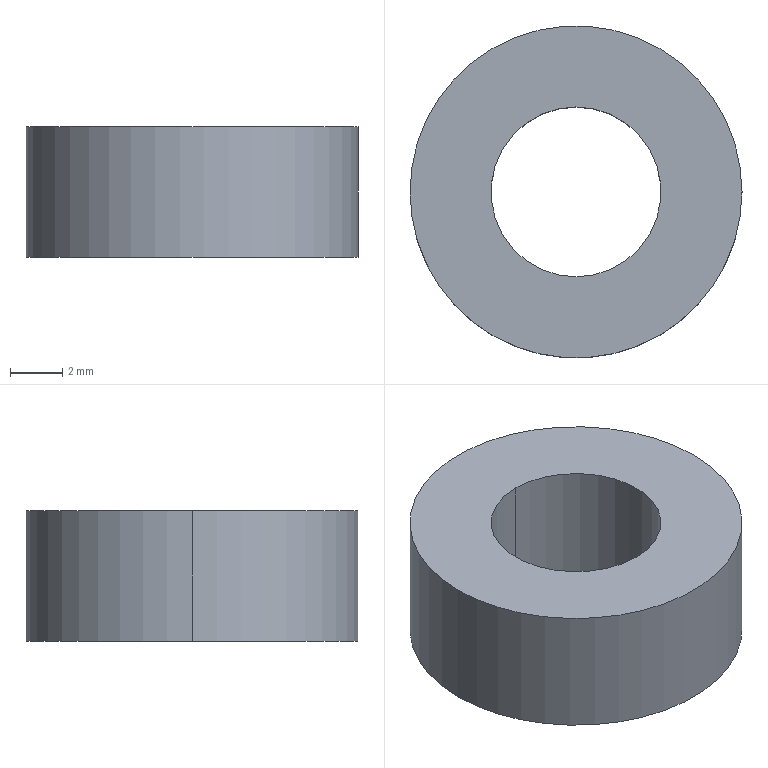Part | STEP file | 1_id1470_x_t | 1 solid | 6 faces | box 12.7 x 12.7 x 5 mm | volume 467.469 mm3 | cylinder 4 | plane 2 | commonest cylinder face diameters 6.5 x2 12.7 x2
STEP:
#1=CARTESIAN_POINT('',(0.,0.,0.));
#2=DIRECTION('',(0.,0.,1.));
#3=DIRECTION('',(1.,0.,0.));
#4=AXIS2_PLACEMENT_3D('',#1,#2,#3);
#5=CARTESIAN_POINT('',(928.809,131.395,-85.));
#6=VERTEX_POINT('',#5);
#7=CARTESIAN_POINT('',(928.809,137.895,-85.));
#8=VERTEX_POINT('',#7);
#9=CARTESIAN_POINT('',(928.809,134.645,-85.));
#10=DIRECTION('',(0.,0.,1.));
#11=DIRECTION('',(0.,-1.,0.));
#12=AXIS2_PLACEMENT_3D('',#9,#10,#11);
#13=CIRCLE('',#12,3.25);
#14=CARTESIAN_POINT('',(928.809,134.645,-88.25));
#15=DIRECTION('',(0.,0.,-1.));
#16=DIRECTION('',(0.,-1.,0.));
#17=AXIS2_PLACEMENT_3D('',#14,#15,#16);
#18=CYLINDRICAL_SURFACE('',#17,3.25);
#19=CARTESIAN_POINT('',(6.283,-3.25));
#20=DIRECTION('',(-1.,0.));
#21=VECTOR('',#20,1.);
#22=LINE('',#19,#21);
#23=(GEOMETRIC_REPRESENTATION_CONTEXT(2)PARAMETRIC_REPRESENTATION_CONTEXT()REPRESENTATION_CONTEXT('',''));
#24=DEFINITIONAL_REPRESENTATION('',(#22),#23);
#25=PCURVE('',#18,#24);
#26=CARTESIAN_POINT('',(928.809,134.645,-85.));
#27=DIRECTION('',(0.,0.,1.));
#28=DIRECTION('',(0.,-1.,0.));
#29=AXIS2_PLACEMENT_3D('',#26,#27,#28);
#30=PLANE('',#29);
#31=CARTESIAN_POINT('',(0.,0.));
#32=DIRECTION('',(1.,0.));
#33=AXIS2_PLACEMENT_2D('',#31,#32);
#34=CIRCLE('',#33,3.25);
#35=(GEOMETRIC_REPRESENTATION_CONTEXT(2)PARAMETRIC_REPRESENTATION_CONTEXT()REPRESENTATION_CONTEXT('',''));
#36=DEFINITIONAL_REPRESENTATION('',(#34),#35);
#37=PCURVE('',#30,#36);
#38=SURFACE_CURVE('',#13,(#25,#37),.PCURVE_S1.);
#39=EDGE_CURVE('',#6,#8,#38,.T.);
#40=ORIENTED_EDGE('',*,*,#39,.T.);
#41=CARTESIAN_POINT('',(928.809,137.895,-80.));
#42=VERTEX_POINT('',#41);
#43=CARTESIAN_POINT('',(928.809,137.895,-80.));
#44=DIRECTION('',(0.,0.,1.));
#45=VECTOR('',#44,1.);
#46=LINE('',#43,#45);
#47=CARTESIAN_POINT('',(3.142,-8.25));
#48=DIRECTION('',(0.,-1.));
#49=VECTOR('',#48,1.);
#50=LINE('',#47,#49);
#51=(GEOMETRIC_REPRESENTATION_CONTEXT(2)PARAMETRIC_REPRESENTATION_CONTEXT()REPRESENTATION_CONTEXT('',''));
#52=DEFINITIONAL_REPRESENTATION('',(#50),#51);
#53=PCURVE('',#18,#52);
#54=CARTESIAN_POINT('',(928.809,134.645,-88.25));
#55=DIRECTION('',(0.,0.,-1.));
#56=DIRECTION('',(0.,-1.,0.));
#57=AXIS2_PLACEMENT_3D('',#54,#55,#56);
#58=CYLINDRICAL_SURFACE('',#57,3.25);
#59=CARTESIAN_POINT('',(3.142,-8.25));
#60=DIRECTION('',(0.,-1.));
#61=VECTOR('',#60,1.);
#62=LINE('',#59,#61);
#63=(GEOMETRIC_REPRESENTATION_CONTEXT(2)PARAMETRIC_REPRESENTATION_CONTEXT()REPRESENTATION_CONTEXT('',''));
#64=DEFINITIONAL_REPRESENTATION('',(#62),#63);
#65=PCURVE('',#58,#64);
#66=SURFACE_CURVE('',#46,(#53,#65),.PCURVE_S1.);
#67=EDGE_CURVE('',#8,#42,#66,.T.);
#68=ORIENTED_EDGE('',*,*,#67,.T.);
#69=CARTESIAN_POINT('',(928.809,131.395,-80.));
#70=VERTEX_POINT('',#69);
#71=CARTESIAN_POINT('',(928.809,134.645,-80.));
#72=DIRECTION('',(0.,0.,-1.));
#73=DIRECTION('',(0.,1.,0.));
#74=AXIS2_PLACEMENT_3D('',#71,#72,#73);
#75=CIRCLE('',#74,3.25);
#76=CARTESIAN_POINT('',(3.142,-8.25));
#77=DIRECTION('',(1.,0.));
#78=VECTOR('',#77,1.);
#79=LINE('',#76,#78);
#80=(GEOMETRIC_REPRESENTATION_CONTEXT(2)PARAMETRIC_REPRESENTATION_CONTEXT()REPRESENTATION_CONTEXT('',''));
#81=DEFINITIONAL_REPRESENTATION('',(#79),#80);
#82=PCURVE('',#18,#81);
#83=CARTESIAN_POINT('',(928.809,134.645,-80.));
#84=DIRECTION('',(0.,0.,1.));
#85=DIRECTION('',(0.,-1.,0.));
#86=AXIS2_PLACEMENT_3D('',#83,#84,#85);
#87=PLANE('',#86);
#88=CARTESIAN_POINT('',(-3.25,0.));
#89=CARTESIAN_POINT('',(-3.25,5.629));
#90=CARTESIAN_POINT('',(1.625,2.815));
#91=CARTESIAN_POINT('',(6.5,0.));
#92=CARTESIAN_POINT('',(1.625,-2.815));
#93=CARTESIAN_POINT('',(-3.25,-5.629));
#94=CARTESIAN_POINT('',(-3.25,0.));
#95=(BOUNDED_CURVE()B_SPLINE_CURVE(2,(#88,#89,#90,#91,#92,#93,#94),.UNSPECIFIED.,.T.,.F.)B_SPLINE_CURVE_WITH_KNOTS((1,2,2,2,2,1),(-2.094,0.,2.094,4.189,6.283,8.378),.UNSPECIFIED.)CURVE()GEOMETRIC_REPRESENTATION_ITEM()RATIONAL_B_SPLINE_CURVE((1.,0.5,1.,0.5,1.,0.5,1.))REPRESENTATION_ITEM(''));
#96=(GEOMETRIC_REPRESENTATION_CONTEXT(2)PARAMETRIC_REPRESENTATION_CONTEXT()REPRESENTATION_CONTEXT('',''));
#97=DEFINITIONAL_REPRESENTATION('',(#95),#96);
#98=PCURVE('',#87,#97);
#99=SURFACE_CURVE('',#75,(#82,#98),.PCURVE_S1.);
#100=EDGE_CURVE('',#42,#70,#99,.T.);
#101=ORIENTED_EDGE('',*,*,#100,.T.);
#102=CARTESIAN_POINT('',(928.809,131.395,-80.));
#103=DIRECTION('',(0.,0.,-1.));
#104=VECTOR('',#103,1.);
#105=LINE('',#102,#104);
#106=CARTESIAN_POINT('',(6.283,-8.25));
#107=DIRECTION('',(0.,1.));
#108=VECTOR('',#107,1.);
#109=LINE('',#106,#108);
#110=(GEOMETRIC_REPRESENTATION_CONTEXT(2)PARAMETRIC_REPRESENTATION_CONTEXT()REPRESENTATION_CONTEXT('',''));
#111=DEFINITIONAL_REPRESENTATION('',(#109),#110);
#112=PCURVE('',#18,#111);
#113=CARTESIAN_POINT('',(0.,-8.25));
#114=DIRECTION('',(0.,1.));
#115=VECTOR('',#114,1.);
#116=LINE('',#113,#115);
#117=(GEOMETRIC_REPRESENTATION_CONTEXT(2)PARAMETRIC_REPRESENTATION_CONTEXT()REPRESENTATION_CONTEXT('',''));
#118=DEFINITIONAL_REPRESENTATION('',(#116),#117);
#119=PCURVE('',#58,#118);
#120=SURFACE_CURVE('',#105,(#112,#119),.PCURVE_S1.);
#121=EDGE_CURVE('',#70,#6,#120,.T.);
#122=ORIENTED_EDGE('',*,*,#121,.T.);
#123=EDGE_LOOP('',(#40,#68,#101,#122));
#124=FACE_BOUND('',#123,.F.);
#125=ADVANCED_FACE('',(#124),#18,.F.);
#126=CARTESIAN_POINT('',(922.459,134.645,-85.));
#127=VERTEX_POINT('',#126);
#128=CARTESIAN_POINT('',(935.159,134.645,-85.));
#129=VERTEX_POINT('',#128);
#130=CARTESIAN_POINT('',(928.809,134.645,-85.));
#131=DIRECTION('',(0.,0.,-1.));
#132=DIRECTION('',(-1.,0.,0.));
#133=AXIS2_PLACEMENT_3D('',#130,#131,#132);
#134=CIRCLE('',#133,6.35);
#135=CARTESIAN_POINT('',(0.,-6.35));
#136=CARTESIAN_POINT('',(-10.999,-6.35));
#137=CARTESIAN_POINT('',(-5.499,3.175));
#138=CARTESIAN_POINT('',(0.,12.7));
#139=CARTESIAN_POINT('',(5.499,3.175));
#140=CARTESIAN_POINT('',(10.999,-6.35));
#141=CARTESIAN_POINT('',(0.,-6.35));
#142=(BOUNDED_CURVE()B_SPLINE_CURVE(2,(#135,#136,#137,#138,#139,#140,#141),.UNSPECIFIED.,.T.,.F.)B_SPLINE_CURVE_WITH_KNOTS((1,2,2,2,2,1),(-2.094,0.,2.094,4.189,6.283,8.378),.UNSPECIFIED.)CURVE()GEOMETRIC_REPRESENTATION_ITEM()RATIONAL_B_SPLINE_CURVE((1.,0.5,1.,0.5,1.,0.5,1.))REPRESENTATION_ITEM(''));
#143=(GEOMETRIC_REPRESENTATION_CONTEXT(2)PARAMETRIC_REPRESENTATION_CONTEXT()REPRESENTATION_CONTEXT('',''));
#144=DEFINITIONAL_REPRESENTATION('',(#142),#143);
#145=PCURVE('',#30,#144);
#146=CARTESIAN_POINT('',(928.809,134.645,-80.));
#147=DIRECTION('',(0.,0.,1.));
#148=DIRECTION('',(1.,0.,0.));
#149=AXIS2_PLACEMENT_3D('',#146,#147,#148);
#150=CYLINDRICAL_SURFACE('',#149,6.35);
#151=CARTESIAN_POINT('',(3.142,-5.));
#152=DIRECTION('',(-1.,0.));
#153=VECTOR('',#152,1.);
#154=LINE('',#151,#153);
#155=(GEOMETRIC_REPRESENTATION_CONTEXT(2)PARAMETRIC_REPRESENTATION_CONTEXT()REPRESENTATION_CONTEXT('',''));
#156=DEFINITIONAL_REPRESENTATION('',(#154),#155);
#157=PCURVE('',#150,#156);
#158=SURFACE_CURVE('',#134,(#145,#157),.PCURVE_S1.);
#159=EDGE_CURVE('',#127,#129,#158,.T.);
#160=ORIENTED_EDGE('',*,*,#159,.T.);
#161=CARTESIAN_POINT('',(928.809,134.645,-85.));
#162=DIRECTION('',(0.,0.,-1.));
#163=DIRECTION('',(1.,0.,0.));
#164=AXIS2_PLACEMENT_3D('',#161,#162,#163);
#165=CIRCLE('',#164,6.35);
#166=CARTESIAN_POINT('',(0.,6.35));
#167=CARTESIAN_POINT('',(10.999,6.35));
#168=CARTESIAN_POINT('',(5.499,-3.175));
#169=CARTESIAN_POINT('',(0.,-12.7));
#170=CARTESIAN_POINT('',(-5.499,-3.175));
#171=CARTESIAN_POINT('',(-10.999,6.35));
#172=CARTESIAN_POINT('',(0.,6.35));
#173=(BOUNDED_CURVE()B_SPLINE_CURVE(2,(#166,#167,#168,#169,#170,#171,#172),.UNSPECIFIED.,.T.,.F.)B_SPLINE_CURVE_WITH_KNOTS((1,2,2,2,2,1),(-2.094,0.,2.094,4.189,6.283,8.378),.UNSPECIFIED.)CURVE()GEOMETRIC_REPRESENTATION_ITEM()RATIONAL_B_SPLINE_CURVE((1.,0.5,1.,0.5,1.,0.5,1.))REPRESENTATION_ITEM(''));
#174=(GEOMETRIC_REPRESENTATION_CONTEXT(2)PARAMETRIC_REPRESENTATION_CONTEXT()REPRESENTATION_CONTEXT('',''));
#175=DEFINITIONAL_REPRESENTATION('',(#173),#174);
#176=PCURVE('',#30,#175);
#177=CARTESIAN_POINT('',(928.809,134.645,-80.));
#178=DIRECTION('',(0.,0.,1.));
#179=DIRECTION('',(1.,0.,0.));
#180=AXIS2_PLACEMENT_3D('',#177,#178,#179);
#181=CYLINDRICAL_SURFACE('',#180,6.35);
#182=CARTESIAN_POINT('',(6.283,-5.));
#183=DIRECTION('',(-1.,0.));
#184=VECTOR('',#183,1.);
#185=LINE('',#182,#184);
#186=(GEOMETRIC_REPRESENTATION_CONTEXT(2)PARAMETRIC_REPRESENTATION_CONTEXT()REPRESENTATION_CONTEXT('',''));
#187=DEFINITIONAL_REPRESENTATION('',(#185),#186);
#188=PCURVE('',#181,#187);
#189=SURFACE_CURVE('',#165,(#176,#188),.PCURVE_S1.);
#190=EDGE_CURVE('',#129,#127,#189,.T.);
#191=ORIENTED_EDGE('',*,*,#190,.T.);
#192=EDGE_LOOP('',(#160,#191));
#193=FACE_BOUND('',#192,.T.);
#194=ORIENTED_EDGE('',*,*,#39,.T.);
#195=CARTESIAN_POINT('',(928.809,134.645,-85.));
#196=DIRECTION('',(0.,0.,1.));
#197=DIRECTION('',(0.,1.,0.));
#198=AXIS2_PLACEMENT_3D('',#195,#196,#197);
#199=CIRCLE('',#198,3.25);
#200=CARTESIAN_POINT('',(0.,0.));
#201=DIRECTION('',(-1.,0.));
#202=AXIS2_PLACEMENT_2D('',#200,#201);
#203=CIRCLE('',#202,3.25);
#204=(GEOMETRIC_REPRESENTATION_CONTEXT(2)PARAMETRIC_REPRESENTATION_CONTEXT()REPRESENTATION_CONTEXT('',''));
#205=DEFINITIONAL_REPRESENTATION('',(#203),#204);
#206=PCURVE('',#30,#205);
#207=CARTESIAN_POINT('',(3.142,-3.25));
#208=DIRECTION('',(-1.,0.));
#209=VECTOR('',#208,1.);
#210=LINE('',#207,#209);
#211=(GEOMETRIC_REPRESENTATION_CONTEXT(2)PARAMETRIC_REPRESENTATION_CONTEXT()REPRESENTATION_CONTEXT('',''));
#212=DEFINITIONAL_REPRESENTATION('',(#210),#211);
#213=PCURVE('',#58,#212);
#214=SURFACE_CURVE('',#199,(#206,#213),.PCURVE_S1.);
#215=EDGE_CURVE('',#8,#6,#214,.T.);
#216=ORIENTED_EDGE('',*,*,#215,.T.);
#217=EDGE_LOOP('',(#194,#216));
#218=FACE_BOUND('',#217,.T.);
#219=ADVANCED_FACE('',(#193,#218),#30,.F.);
#220=CARTESIAN_POINT('',(935.159,134.645,-80.));
#221=VERTEX_POINT('',#220);
#222=CARTESIAN_POINT('',(935.159,134.645,-85.));
#223=DIRECTION('',(0.,0.,-1.));
#224=VECTOR('',#223,1.);
#225=LINE('',#222,#224);
#226=CARTESIAN_POINT('',(6.283,-5.));
#227=DIRECTION('',(0.,-1.));
#228=VECTOR('',#227,1.);
#229=LINE('',#226,#228);
#230=(GEOMETRIC_REPRESENTATION_CONTEXT(2)PARAMETRIC_REPRESENTATION_CONTEXT()REPRESENTATION_CONTEXT('',''));
#231=DEFINITIONAL_REPRESENTATION('',(#229),#230);
#232=PCURVE('',#181,#231);
#233=CARTESIAN_POINT('',(0.,-5.));
#234=DIRECTION('',(0.,-1.));
#235=VECTOR('',#234,1.);
#236=LINE('',#233,#235);
#237=(GEOMETRIC_REPRESENTATION_CONTEXT(2)PARAMETRIC_REPRESENTATION_CONTEXT()REPRESENTATION_CONTEXT('',''));
#238=DEFINITIONAL_REPRESENTATION('',(#236),#237);
#239=PCURVE('',#150,#238);
#240=SURFACE_CURVE('',#225,(#232,#239),.PCURVE_S1.);
#241=EDGE_CURVE('',#221,#129,#240,.T.);
#242=ORIENTED_EDGE('',*,*,#241,.F.);
#243=CARTESIAN_POINT('',(922.459,134.645,-80.));
#244=VERTEX_POINT('',#243);
#245=CARTESIAN_POINT('',(928.809,134.645,-80.));
#246=DIRECTION('',(0.,0.,1.));
#247=DIRECTION('',(-1.,0.,0.));
#248=AXIS2_PLACEMENT_3D('',#245,#246,#247);
#249=CIRCLE('',#248,6.35);
#250=CARTESIAN_POINT('',(3.142,0.));
#251=DIRECTION('',(1.,0.));
#252=VECTOR('',#251,1.);
#253=LINE('',#250,#252);
#254=(GEOMETRIC_REPRESENTATION_CONTEXT(2)PARAMETRIC_REPRESENTATION_CONTEXT()REPRESENTATION_CONTEXT('',''));
#255=DEFINITIONAL_REPRESENTATION('',(#253),#254);
#256=PCURVE('',#181,#255);
#257=CARTESIAN_POINT('',(0.,0.));
#258=DIRECTION('',(0.,-1.));
#259=AXIS2_PLACEMENT_2D('',#257,#258);
#260=CIRCLE('',#259,6.35);
#261=(GEOMETRIC_REPRESENTATION_CONTEXT(2)PARAMETRIC_REPRESENTATION_CONTEXT()REPRESENTATION_CONTEXT('',''));
#262=DEFINITIONAL_REPRESENTATION('',(#260),#261);
#263=PCURVE('',#87,#262);
#264=SURFACE_CURVE('',#249,(#256,#263),.PCURVE_S1.);
#265=EDGE_CURVE('',#244,#221,#264,.T.);
#266=ORIENTED_EDGE('',*,*,#265,.F.);
#267=CARTESIAN_POINT('',(922.459,134.645,-85.));
#268=DIRECTION('',(0.,0.,1.));
#269=VECTOR('',#268,1.);
#270=LINE('',#267,#269);
#271=CARTESIAN_POINT('',(3.142,-5.));
#272=DIRECTION('',(0.,1.));
#273=VECTOR('',#272,1.);
#274=LINE('',#271,#273);
#275=(GEOMETRIC_REPRESENTATION_CONTEXT(2)PARAMETRIC_REPRESENTATION_CONTEXT()REPRESENTATION_CONTEXT('',''));
#276=DEFINITIONAL_REPRESENTATION('',(#274),#275);
#277=PCURVE('',#181,#276);
#278=CARTESIAN_POINT('',(3.142,-5.));
#279=DIRECTION('',(0.,1.));
#280=VECTOR('',#279,1.);
#281=LINE('',#278,#280);
#282=(GEOMETRIC_REPRESENTATION_CONTEXT(2)PARAMETRIC_REPRESENTATION_CONTEXT()REPRESENTATION_CONTEXT('',''));
#283=DEFINITIONAL_REPRESENTATION('',(#281),#282);
#284=PCURVE('',#150,#283);
#285=SURFACE_CURVE('',#270,(#277,#284),.PCURVE_S1.);
#286=EDGE_CURVE('',#127,#244,#285,.T.);
#287=ORIENTED_EDGE('',*,*,#286,.F.);
#288=ORIENTED_EDGE('',*,*,#190,.F.);
#289=EDGE_LOOP('',(#242,#266,#287,#288));
#290=FACE_BOUND('',#289,.T.);
#291=ADVANCED_FACE('',(#290),#181,.T.);
#292=ORIENTED_EDGE('',*,*,#286,.T.);
#293=CARTESIAN_POINT('',(928.809,134.645,-80.));
#294=DIRECTION('',(0.,0.,1.));
#295=DIRECTION('',(1.,0.,0.));
#296=AXIS2_PLACEMENT_3D('',#293,#294,#295);
#297=CIRCLE('',#296,6.35);
#298=CARTESIAN_POINT('',(0.,0.));
#299=DIRECTION('',(1.,0.));
#300=VECTOR('',#299,1.);
#301=LINE('',#298,#300);
#302=(GEOMETRIC_REPRESENTATION_CONTEXT(2)PARAMETRIC_REPRESENTATION_CONTEXT()REPRESENTATION_CONTEXT('',''));
#303=DEFINITIONAL_REPRESENTATION('',(#301),#302);
#304=PCURVE('',#150,#303);
#305=CARTESIAN_POINT('',(0.,0.));
#306=DIRECTION('',(0.,1.));
#307=AXIS2_PLACEMENT_2D('',#305,#306);
#308=CIRCLE('',#307,6.35);
#309=(GEOMETRIC_REPRESENTATION_CONTEXT(2)PARAMETRIC_REPRESENTATION_CONTEXT()REPRESENTATION_CONTEXT('',''));
#310=DEFINITIONAL_REPRESENTATION('',(#308),#309);
#311=PCURVE('',#87,#310);
#312=SURFACE_CURVE('',#297,(#304,#311),.PCURVE_S1.);
#313=EDGE_CURVE('',#221,#244,#312,.T.);
#314=ORIENTED_EDGE('',*,*,#313,.F.);
#315=ORIENTED_EDGE('',*,*,#241,.T.);
#316=ORIENTED_EDGE('',*,*,#159,.F.);
#317=EDGE_LOOP('',(#292,#314,#315,#316));
#318=FACE_BOUND('',#317,.T.);
#319=ADVANCED_FACE('',(#318),#150,.T.);
#320=ORIENTED_EDGE('',*,*,#265,.T.);
#321=ORIENTED_EDGE('',*,*,#313,.T.);
#322=EDGE_LOOP('',(#320,#321));
#323=FACE_BOUND('',#322,.T.);
#324=CARTESIAN_POINT('',(928.809,134.645,-80.));
#325=DIRECTION('',(0.,0.,-1.));
#326=DIRECTION('',(0.,-1.,0.));
#327=AXIS2_PLACEMENT_3D('',#324,#325,#326);
#328=CIRCLE('',#327,3.25);
#329=CARTESIAN_POINT('',(3.25,0.));
#330=CARTESIAN_POINT('',(3.25,-5.629));
#331=CARTESIAN_POINT('',(-1.625,-2.815));
#332=CARTESIAN_POINT('',(-6.5,0.));
#333=CARTESIAN_POINT('',(-1.625,2.815));
#334=CARTESIAN_POINT('',(3.25,5.629));
#335=CARTESIAN_POINT('',(3.25,0.));
#336=(BOUNDED_CURVE()B_SPLINE_CURVE(2,(#329,#330,#331,#332,#333,#334,#335),.UNSPECIFIED.,.T.,.F.)B_SPLINE_CURVE_WITH_KNOTS((1,2,2,2,2,1),(-2.094,0.,2.094,4.189,6.283,8.378),.UNSPECIFIED.)CURVE()GEOMETRIC_REPRESENTATION_ITEM()RATIONAL_B_SPLINE_CURVE((1.,0.5,1.,0.5,1.,0.5,1.))REPRESENTATION_ITEM(''));
#337=(GEOMETRIC_REPRESENTATION_CONTEXT(2)PARAMETRIC_REPRESENTATION_CONTEXT()REPRESENTATION_CONTEXT('',''));
#338=DEFINITIONAL_REPRESENTATION('',(#336),#337);
#339=PCURVE('',#87,#338);
#340=CARTESIAN_POINT('',(0.,-8.25));
#341=DIRECTION('',(1.,0.));
#342=VECTOR('',#341,1.);
#343=LINE('',#340,#342);
#344=(GEOMETRIC_REPRESENTATION_CONTEXT(2)PARAMETRIC_REPRESENTATION_CONTEXT()REPRESENTATION_CONTEXT('',''));
#345=DEFINITIONAL_REPRESENTATION('',(#343),#344);
#346=PCURVE('',#58,#345);
#347=SURFACE_CURVE('',#328,(#339,#346),.PCURVE_S1.);
#348=EDGE_CURVE('',#70,#42,#347,.T.);
#349=ORIENTED_EDGE('',*,*,#348,.T.);
#350=ORIENTED_EDGE('',*,*,#100,.T.);
#351=EDGE_LOOP('',(#349,#350));
#352=FACE_BOUND('',#351,.T.);
#353=ADVANCED_FACE('',(#323,#352),#87,.T.);
#354=ORIENTED_EDGE('',*,*,#215,.T.);
#355=ORIENTED_EDGE('',*,*,#121,.F.);
#356=ORIENTED_EDGE('',*,*,#348,.T.);
#357=ORIENTED_EDGE('',*,*,#67,.F.);
#358=EDGE_LOOP('',(#354,#355,#356,#357));
#359=FACE_BOUND('',#358,.F.);
#360=ADVANCED_FACE('',(#359),#58,.F.);
#361=CLOSED_SHELL('',(#125,#219,#291,#319,#353,#360));
#362=MANIFOLD_SOLID_BREP('',#361);
#363=(LENGTH_UNIT()NAMED_UNIT(*)SI_UNIT(.MILLI.,.METRE.));
#364=UNCERTAINTY_MEASURE_WITH_UNIT(LENGTH_MEASURE(0.0000001),#363,'','');
#365=(NAMED_UNIT(*)PLANE_ANGLE_UNIT()SI_UNIT($,.RADIAN.));
#366=(NAMED_UNIT(*)SI_UNIT($,.STERADIAN.)SOLID_ANGLE_UNIT());
#367=(GEOMETRIC_REPRESENTATION_CONTEXT(3)GLOBAL_UNCERTAINTY_ASSIGNED_CONTEXT((#364))GLOBAL_UNIT_ASSIGNED_CONTEXT((#363,#365,#366))REPRESENTATION_CONTEXT('',''));
#368=ADVANCED_BREP_SHAPE_REPRESENTATION('',(#4,#362),#367);